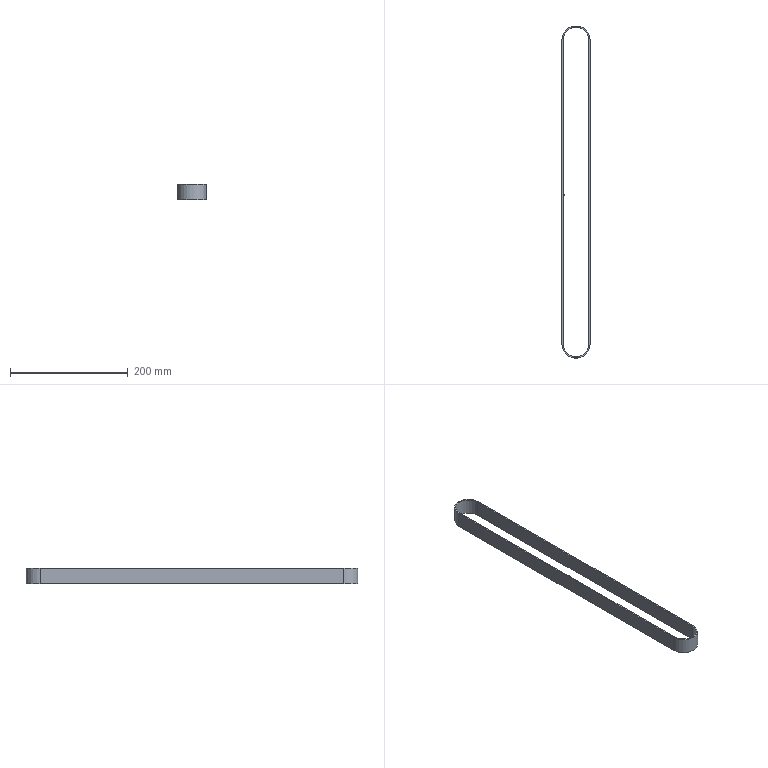Part | SolidWorks | features CompositeCurve 1, Extrusion 1, ICE 1 | 1 solid | 19 faces | box 47.9 x 564.4 x 27 mm | volume 68430 mm3 | cylinder 12 | plane 7 | commonest cylinder face diameters 0.5 x2 1.1 x2 6.55 x2 40.06 x2 43.6 x2 47.9 x2
STEP:
#1=CARTESIAN_POINT('',(-20.121,-262.156,27.));
#2=VERTEX_POINT('',#1);
#3=CARTESIAN_POINT('',(-20.132,-262.842,27.));
#4=VERTEX_POINT('',#3);
#5=CARTESIAN_POINT('',(-0.1024,-262.842,27.));
#6=DIRECTION('',(0.,0.,1.));
#7=DIRECTION('',(-1.,0.,0.));
#8=AXIS2_PLACEMENT_3D('',#5,#6,#7);
#9=CIRCLE('',#8,20.03);
#10=EDGE_CURVE('',#2,#4,#9,.T.);
#11=ORIENTED_EDGE('',*,*,#10,.T.);
#12=CARTESIAN_POINT('',(-20.132,-262.842,0.));
#13=VERTEX_POINT('',#12);
#14=CARTESIAN_POINT('',(-20.132,-262.842,31.346));
#15=DIRECTION('',(0.,0.,-1.));
#16=VECTOR('',#15,1000.);
#17=LINE('',#14,#16);
#18=EDGE_CURVE('',#4,#13,#17,.T.);
#19=ORIENTED_EDGE('',*,*,#18,.T.);
#20=CARTESIAN_POINT('',(-20.121,-262.156,0.));
#21=VERTEX_POINT('',#20);
#22=CARTESIAN_POINT('',(-0.1024,-262.842,0.));
#23=DIRECTION('',(0.,0.,-1.));
#24=DIRECTION('',(1.,0.,0.));
#25=AXIS2_PLACEMENT_3D('',#22,#23,#24);
#26=CIRCLE('',#25,20.03);
#27=EDGE_CURVE('',#13,#21,#26,.T.);
#28=ORIENTED_EDGE('',*,*,#27,.T.);
#29=CARTESIAN_POINT('',(-20.121,-262.156,31.346));
#30=DIRECTION('',(0.,0.,-1.));
#31=VECTOR('',#30,1000.);
#32=LINE('',#29,#31);
#33=EDGE_CURVE('',#2,#21,#32,.T.);
#34=ORIENTED_EDGE('',*,*,#33,.F.);
#35=EDGE_LOOP('',(#11,#19,#28,#34));
#36=FACE_OUTER_BOUND('',#35,.T.);
#37=CARTESIAN_POINT('',(-0.1024,-262.842,31.346));
#38=DIRECTION('',(0.,0.,-1.));
#39=DIRECTION('',(-1.,0.,0.));
#40=AXIS2_PLACEMENT_3D('',#37,#38,#39);
#41=CYLINDRICAL_SURFACE('',#40,20.03);
#42=ADVANCED_FACE('',(#36),#41,.F.);
#43=CARTESIAN_POINT('',(-21.8,-260.838,27.));
#44=VERTEX_POINT('',#43);
#45=CARTESIAN_POINT('',(-21.8,0.,27.));
#46=VERTEX_POINT('',#45);
#47=CARTESIAN_POINT('',(-21.8,-516.5,27.));
#48=DIRECTION('',(0.,1.,0.));
#49=VECTOR('',#48,1000.);
#50=LINE('',#47,#49);
#51=EDGE_CURVE('',#44,#46,#50,.T.);
#52=ORIENTED_EDGE('',*,*,#51,.F.);
#53=CARTESIAN_POINT('',(-21.8,-260.838,0.));
#54=VERTEX_POINT('',#53);
#55=CARTESIAN_POINT('',(-21.8,-260.838,31.346));
#56=DIRECTION('',(0.,0.,-1.));
#57=VECTOR('',#56,1000.);
#58=LINE('',#55,#57);
#59=EDGE_CURVE('',#44,#54,#58,.T.);
#60=ORIENTED_EDGE('',*,*,#59,.T.);
#61=CARTESIAN_POINT('',(-21.8,0.,0.));
#62=VERTEX_POINT('',#61);
#63=CARTESIAN_POINT('',(-21.8,-516.5,0.));
#64=DIRECTION('',(0.,-1.,0.));
#65=VECTOR('',#64,1000.);
#66=LINE('',#63,#65);
#67=EDGE_CURVE('',#62,#54,#66,.T.);
#68=ORIENTED_EDGE('',*,*,#67,.F.);
#69=CARTESIAN_POINT('',(-21.8,0.,593.429));
#70=DIRECTION('',(0.,0.,-1.));
#71=VECTOR('',#70,1000.);
#72=LINE('',#69,#71);
#73=EDGE_CURVE('',#46,#62,#72,.T.);
#74=ORIENTED_EDGE('',*,*,#73,.F.);
#75=EDGE_LOOP('',(#52,#60,#68,#74));
#76=FACE_OUTER_BOUND('',#75,.T.);
#77=CARTESIAN_POINT('',(-21.8,-516.5,593.429));
#78=DIRECTION('',(1.,0.,0.));
#79=DIRECTION('',(0.,0.,-1.));
#80=AXIS2_PLACEMENT_3D('',#77,#78,#79);
#81=PLANE('',#80);
#82=ADVANCED_FACE('',(#76),#81,.T.);
#83=CARTESIAN_POINT('',(-21.8,-264.847,0.));
#84=VERTEX_POINT('',#83);
#85=CARTESIAN_POINT('',(-21.8,-516.5,0.));
#86=VERTEX_POINT('',#85);
#87=CARTESIAN_POINT('',(-21.8,-516.5,0.));
#88=DIRECTION('',(0.,-1.,0.));
#89=VECTOR('',#88,1000.);
#90=LINE('',#87,#89);
#91=EDGE_CURVE('',#84,#86,#90,.T.);
#92=ORIENTED_EDGE('',*,*,#91,.F.);
#93=CARTESIAN_POINT('',(-21.8,-264.847,27.));
#94=VERTEX_POINT('',#93);
#95=CARTESIAN_POINT('',(-21.8,-264.847,31.346));
#96=DIRECTION('',(0.,0.,-1.));
#97=VECTOR('',#96,1000.);
#98=LINE('',#95,#97);
#99=EDGE_CURVE('',#94,#84,#98,.T.);
#100=ORIENTED_EDGE('',*,*,#99,.F.);
#101=CARTESIAN_POINT('',(-21.8,-516.5,27.));
#102=VERTEX_POINT('',#101);
#103=CARTESIAN_POINT('',(-21.8,-516.5,27.));
#104=DIRECTION('',(0.,1.,0.));
#105=VECTOR('',#104,1000.);
#106=LINE('',#103,#105);
#107=EDGE_CURVE('',#102,#94,#106,.T.);
#108=ORIENTED_EDGE('',*,*,#107,.F.);
#109=CARTESIAN_POINT('',(-21.8,-516.5,593.429));
#110=DIRECTION('',(0.,0.,-1.));
#111=VECTOR('',#110,1000.);
#112=LINE('',#109,#111);
#113=EDGE_CURVE('',#102,#86,#112,.T.);
#114=ORIENTED_EDGE('',*,*,#113,.T.);
#115=EDGE_LOOP('',(#92,#100,#108,#114));
#116=FACE_OUTER_BOUND('',#115,.T.);
#117=CARTESIAN_POINT('',(-21.8,-516.5,593.429));
#118=DIRECTION('',(1.,0.,0.));
#119=DIRECTION('',(0.,0.,-1.));
#120=AXIS2_PLACEMENT_3D('',#117,#118,#119);
#121=PLANE('',#120);
#122=ADVANCED_FACE('',(#116),#121,.T.);
#123=CARTESIAN_POINT('',(-23.95,-516.5,0.));
#124=VERTEX_POINT('',#123);
#125=CARTESIAN_POINT('',(23.95,-516.5,0.));
#126=VERTEX_POINT('',#125);
#127=CARTESIAN_POINT('',(0.,-516.5,0.));
#128=DIRECTION('',(0.,0.,1.));
#129=DIRECTION('',(1.,0.,0.));
#130=AXIS2_PLACEMENT_3D('',#127,#128,#129);
#131=CIRCLE('',#130,23.95);
#132=EDGE_CURVE('',#124,#126,#131,.T.);
#133=ORIENTED_EDGE('',*,*,#132,.F.);
#134=CARTESIAN_POINT('',(-23.95,0.,0.));
#135=VERTEX_POINT('',#134);
#136=CARTESIAN_POINT('',(-23.95,0.,0.));
#137=DIRECTION('',(0.,-1.,0.));
#138=VECTOR('',#137,1000.);
#139=LINE('',#136,#138);
#140=EDGE_CURVE('',#135,#124,#139,.T.);
#141=ORIENTED_EDGE('',*,*,#140,.F.);
#142=CARTESIAN_POINT('',(23.95,0.,0.));
#143=VERTEX_POINT('',#142);
#144=CARTESIAN_POINT('',(0.,0.,0.));
#145=DIRECTION('',(0.,0.,1.));
#146=DIRECTION('',(1.,0.,0.));
#147=AXIS2_PLACEMENT_3D('',#144,#145,#146);
#148=CIRCLE('',#147,23.95);
#149=EDGE_CURVE('',#143,#135,#148,.T.);
#150=ORIENTED_EDGE('',*,*,#149,.F.);
#151=CARTESIAN_POINT('',(23.95,-516.5,0.));
#152=DIRECTION('',(0.,1.,0.));
#153=VECTOR('',#152,1000.);
#154=LINE('',#151,#153);
#155=EDGE_CURVE('',#126,#143,#154,.T.);
#156=ORIENTED_EDGE('',*,*,#155,.F.);
#157=EDGE_LOOP('',(#133,#141,#150,#156));
#158=FACE_OUTER_BOUND('',#157,.T.);
#159=CARTESIAN_POINT('',(21.8,0.,0.));
#160=VERTEX_POINT('',#159);
#161=CARTESIAN_POINT('',(0.,0.,0.));
#162=DIRECTION('',(0.,0.,1.));
#163=DIRECTION('',(1.,0.,0.));
#164=AXIS2_PLACEMENT_3D('',#161,#162,#163);
#165=CIRCLE('',#164,21.8);
#166=EDGE_CURVE('',#160,#62,#165,.T.);
#167=ORIENTED_EDGE('',*,*,#166,.T.);
#168=ORIENTED_EDGE('',*,*,#67,.T.);
#169=CARTESIAN_POINT('',(-21.407,-261.313,0.));
#170=VERTEX_POINT('',#169);
#171=CARTESIAN_POINT('',(-21.253,-260.785,0.));
#172=DIRECTION('',(0.,0.,-1.));
#173=DIRECTION('',(1.,0.,0.));
#174=AXIS2_PLACEMENT_3D('',#171,#172,#173);
#175=CIRCLE('',#174,0.55);
#176=EDGE_CURVE('',#170,#54,#175,.T.);
#177=ORIENTED_EDGE('',*,*,#176,.F.);
#178=CARTESIAN_POINT('',(-20.209,-261.956,0.));
#179=VERTEX_POINT('',#178);
#180=CARTESIAN_POINT('',(-22.324,-264.457,0.));
#181=DIRECTION('',(0.,0.,-1.));
#182=DIRECTION('',(1.,0.,0.));
#183=AXIS2_PLACEMENT_3D('',#180,#181,#182);
#184=CIRCLE('',#183,3.275);
#185=EDGE_CURVE('',#170,#179,#184,.T.);
#186=ORIENTED_EDGE('',*,*,#185,.T.);
#187=CARTESIAN_POINT('',(-20.371,-262.147,0.));
#188=DIRECTION('',(0.,0.,-1.));
#189=DIRECTION('',(1.,0.,0.));
#190=AXIS2_PLACEMENT_3D('',#187,#188,#189);
#191=CIRCLE('',#190,0.25);
#192=EDGE_CURVE('',#179,#21,#191,.T.);
#193=ORIENTED_EDGE('',*,*,#192,.T.);
#194=ORIENTED_EDGE('',*,*,#27,.F.);
#195=CARTESIAN_POINT('',(-20.121,-263.529,0.));
#196=VERTEX_POINT('',#195);
#197=CARTESIAN_POINT('',(-0.1024,-262.842,0.));
#198=DIRECTION('',(0.,0.,-1.));
#199=DIRECTION('',(1.,0.,0.));
#200=AXIS2_PLACEMENT_3D('',#197,#198,#199);
#201=CIRCLE('',#200,20.03);
#202=EDGE_CURVE('',#196,#13,#201,.T.);
#203=ORIENTED_EDGE('',*,*,#202,.F.);
#204=CARTESIAN_POINT('',(-20.209,-263.729,0.));
#205=VERTEX_POINT('',#204);
#206=CARTESIAN_POINT('',(-20.371,-263.538,0.));
#207=DIRECTION('',(0.,0.,-1.));
#208=DIRECTION('',(1.,0.,0.));
#209=AXIS2_PLACEMENT_3D('',#206,#207,#208);
#210=CIRCLE('',#209,0.25);
#211=EDGE_CURVE('',#196,#205,#210,.T.);
#212=ORIENTED_EDGE('',*,*,#211,.T.);
#213=CARTESIAN_POINT('',(-21.407,-264.372,0.));
#214=VERTEX_POINT('',#213);
#215=CARTESIAN_POINT('',(-22.324,-261.228,0.));
#216=DIRECTION('',(0.,0.,-1.));
#217=DIRECTION('',(1.,0.,0.));
#218=AXIS2_PLACEMENT_3D('',#215,#216,#217);
#219=CIRCLE('',#218,3.275);
#220=EDGE_CURVE('',#205,#214,#219,.T.);
#221=ORIENTED_EDGE('',*,*,#220,.T.);
#222=CARTESIAN_POINT('',(-21.253,-264.9,0.));
#223=DIRECTION('',(0.,0.,-1.));
#224=DIRECTION('',(1.,0.,0.));
#225=AXIS2_PLACEMENT_3D('',#222,#223,#224);
#226=CIRCLE('',#225,0.55);
#227=EDGE_CURVE('',#84,#214,#226,.T.);
#228=ORIENTED_EDGE('',*,*,#227,.F.);
#229=ORIENTED_EDGE('',*,*,#91,.T.);
#230=CARTESIAN_POINT('',(21.8,-516.5,0.));
#231=VERTEX_POINT('',#230);
#232=CARTESIAN_POINT('',(0.,-516.5,0.));
#233=DIRECTION('',(0.,0.,1.));
#234=DIRECTION('',(1.,0.,0.));
#235=AXIS2_PLACEMENT_3D('',#232,#233,#234);
#236=CIRCLE('',#235,21.8);
#237=EDGE_CURVE('',#86,#231,#236,.T.);
#238=ORIENTED_EDGE('',*,*,#237,.T.);
#239=CARTESIAN_POINT('',(21.8,0.,0.));
#240=DIRECTION('',(0.,1.,0.));
#241=VECTOR('',#240,1000.);
#242=LINE('',#239,#241);
#243=EDGE_CURVE('',#231,#160,#242,.T.);
#244=ORIENTED_EDGE('',*,*,#243,.T.);
#245=EDGE_LOOP('',(#167,#168,#177,#186,#193,#194,#203,#212,#221,#228,#229,#238,#244));
#246=FACE_BOUND('',#245,.T.);
#247=CARTESIAN_POINT('',(0.,-516.5,0.));
#248=DIRECTION('',(0.,0.,1.));
#249=DIRECTION('',(1.,0.,0.));
#250=AXIS2_PLACEMENT_3D('',#247,#248,#249);
#251=PLANE('',#250);
#252=ADVANCED_FACE('',(#158,#246),#251,.F.);
#253=CARTESIAN_POINT('',(23.95,-516.5,27.));
#254=VERTEX_POINT('',#253);
#255=CARTESIAN_POINT('',(23.95,-516.5,593.429));
#256=DIRECTION('',(0.,0.,-1.));
#257=VECTOR('',#256,1000.);
#258=LINE('',#255,#257);
#259=EDGE_CURVE('',#254,#126,#258,.T.);
#260=ORIENTED_EDGE('',*,*,#259,.F.);
#261=CARTESIAN_POINT('',(-23.95,-516.5,27.));
#262=VERTEX_POINT('',#261);
#263=CARTESIAN_POINT('',(0.,-516.5,27.));
#264=DIRECTION('',(0.,0.,-1.));
#265=DIRECTION('',(-1.,0.,0.));
#266=AXIS2_PLACEMENT_3D('',#263,#264,#265);
#267=CIRCLE('',#266,23.95);
#268=EDGE_CURVE('',#254,#262,#267,.T.);
#269=ORIENTED_EDGE('',*,*,#268,.T.);
#270=CARTESIAN_POINT('',(-23.95,-516.5,593.429));
#271=DIRECTION('',(0.,0.,-1.));
#272=VECTOR('',#271,1000.);
#273=LINE('',#270,#272);
#274=EDGE_CURVE('',#262,#124,#273,.T.);
#275=ORIENTED_EDGE('',*,*,#274,.T.);
#276=ORIENTED_EDGE('',*,*,#132,.T.);
#277=EDGE_LOOP('',(#260,#269,#275,#276));
#278=FACE_OUTER_BOUND('',#277,.T.);
#279=CARTESIAN_POINT('',(0.,-516.5,593.429));
#280=DIRECTION('',(0.,0.,-1.));
#281=DIRECTION('',(-1.,0.,0.));
#282=AXIS2_PLACEMENT_3D('',#279,#280,#281);
#283=CYLINDRICAL_SURFACE('',#282,23.95);
#284=ADVANCED_FACE('',(#278),#283,.T.);
#285=CARTESIAN_POINT('',(23.95,0.,27.));
#286=VERTEX_POINT('',#285);
#287=CARTESIAN_POINT('',(23.95,0.,593.429));
#288=DIRECTION('',(0.,0.,-1.));
#289=VECTOR('',#288,1000.);
#290=LINE('',#287,#289);
#291=EDGE_CURVE('',#286,#143,#290,.T.);
#292=ORIENTED_EDGE('',*,*,#291,.F.);
#293=CARTESIAN_POINT('',(23.95,-516.5,27.));
#294=DIRECTION('',(0.,-1.,0.));
#295=VECTOR('',#294,1000.);
#296=LINE('',#293,#295);
#297=EDGE_CURVE('',#286,#254,#296,.T.);
#298=ORIENTED_EDGE('',*,*,#297,.T.);
#299=ORIENTED_EDGE('',*,*,#259,.T.);
#300=ORIENTED_EDGE('',*,*,#155,.T.);
#301=EDGE_LOOP('',(#292,#298,#299,#300));
#302=FACE_OUTER_BOUND('',#301,.T.);
#303=CARTESIAN_POINT('',(23.95,-516.5,593.429));
#304=DIRECTION('',(-1.,0.,0.));
#305=DIRECTION('',(0.,-1.,0.));
#306=AXIS2_PLACEMENT_3D('',#303,#304,#305);
#307=PLANE('',#306);
#308=ADVANCED_FACE('',(#302),#307,.F.);
#309=CARTESIAN_POINT('',(-23.95,0.,27.));
#310=VERTEX_POINT('',#309);
#311=CARTESIAN_POINT('',(-23.95,0.,593.429));
#312=DIRECTION('',(0.,0.,-1.));
#313=VECTOR('',#312,1000.);
#314=LINE('',#311,#313);
#315=EDGE_CURVE('',#310,#135,#314,.T.);
#316=ORIENTED_EDGE('',*,*,#315,.F.);
#317=CARTESIAN_POINT('',(0.,0.,27.));
#318=DIRECTION('',(0.,0.,-1.));
#319=DIRECTION('',(-1.,0.,0.));
#320=AXIS2_PLACEMENT_3D('',#317,#318,#319);
#321=CIRCLE('',#320,23.95);
#322=EDGE_CURVE('',#310,#286,#321,.T.);
#323=ORIENTED_EDGE('',*,*,#322,.T.);
#324=ORIENTED_EDGE('',*,*,#291,.T.);
#325=ORIENTED_EDGE('',*,*,#149,.T.);
#326=EDGE_LOOP('',(#316,#323,#324,#325));
#327=FACE_OUTER_BOUND('',#326,.T.);
#328=CARTESIAN_POINT('',(0.,0.,593.429));
#329=DIRECTION('',(0.,0.,-1.));
#330=DIRECTION('',(-1.,0.,0.));
#331=AXIS2_PLACEMENT_3D('',#328,#329,#330);
#332=CYLINDRICAL_SURFACE('',#331,23.95);
#333=ADVANCED_FACE('',(#327),#332,.T.);
#334=ORIENTED_EDGE('',*,*,#274,.F.);
#335=CARTESIAN_POINT('',(-23.95,0.,27.));
#336=DIRECTION('',(0.,1.,0.));
#337=VECTOR('',#336,1000.);
#338=LINE('',#335,#337);
#339=EDGE_CURVE('',#262,#310,#338,.T.);
#340=ORIENTED_EDGE('',*,*,#339,.T.);
#341=ORIENTED_EDGE('',*,*,#315,.T.);
#342=ORIENTED_EDGE('',*,*,#140,.T.);
#343=EDGE_LOOP('',(#334,#340,#341,#342));
#344=FACE_OUTER_BOUND('',#343,.T.);
#345=CARTESIAN_POINT('',(-23.95,0.,593.429));
#346=DIRECTION('',(1.,0.,0.));
#347=DIRECTION('',(0.,1.,0.));
#348=AXIS2_PLACEMENT_3D('',#345,#346,#347);
#349=PLANE('',#348);
#350=ADVANCED_FACE('',(#344),#349,.F.);
#351=CARTESIAN_POINT('',(21.8,0.,27.));
#352=VERTEX_POINT('',#351);
#353=CARTESIAN_POINT('',(0.,0.,27.));
#354=DIRECTION('',(0.,0.,-1.));
#355=DIRECTION('',(-1.,0.,0.));
#356=AXIS2_PLACEMENT_3D('',#353,#354,#355);
#357=CIRCLE('',#356,21.8);
#358=EDGE_CURVE('',#46,#352,#357,.T.);
#359=ORIENTED_EDGE('',*,*,#358,.F.);
#360=ORIENTED_EDGE('',*,*,#73,.T.);
#361=ORIENTED_EDGE('',*,*,#166,.F.);
#362=CARTESIAN_POINT('',(21.8,0.,593.429));
#363=DIRECTION('',(0.,0.,-1.));
#364=VECTOR('',#363,1000.);
#365=LINE('',#362,#364);
#366=EDGE_CURVE('',#352,#160,#365,.T.);
#367=ORIENTED_EDGE('',*,*,#366,.F.);
#368=EDGE_LOOP('',(#359,#360,#361,#367));
#369=FACE_OUTER_BOUND('',#368,.T.);
#370=CARTESIAN_POINT('',(0.,0.,593.429));
#371=DIRECTION('',(0.,0.,-1.));
#372=DIRECTION('',(-1.,0.,0.));
#373=AXIS2_PLACEMENT_3D('',#370,#371,#372);
#374=CYLINDRICAL_SURFACE('',#373,21.8);
#375=ADVANCED_FACE('',(#369),#374,.F.);
#376=CARTESIAN_POINT('',(21.8,-516.5,27.));
#377=VERTEX_POINT('',#376);
#378=CARTESIAN_POINT('',(0.,-516.5,27.));
#379=DIRECTION('',(0.,0.,-1.));
#380=DIRECTION('',(-1.,0.,0.));
#381=AXIS2_PLACEMENT_3D('',#378,#379,#380);
#382=CIRCLE('',#381,21.8);
#383=EDGE_CURVE('',#377,#102,#382,.T.);
#384=ORIENTED_EDGE('',*,*,#383,.F.);
#385=CARTESIAN_POINT('',(21.8,-516.5,593.429));
#386=DIRECTION('',(0.,0.,-1.));
#387=VECTOR('',#386,1000.);
#388=LINE('',#385,#387);
#389=EDGE_CURVE('',#377,#231,#388,.T.);
#390=ORIENTED_EDGE('',*,*,#389,.T.);
#391=ORIENTED_EDGE('',*,*,#237,.F.);
#392=ORIENTED_EDGE('',*,*,#113,.F.);
#393=EDGE_LOOP('',(#384,#390,#391,#392));
#394=FACE_OUTER_BOUND('',#393,.T.);
#395=CARTESIAN_POINT('',(0.,-516.5,593.429));
#396=DIRECTION('',(0.,0.,-1.));
#397=DIRECTION('',(-1.,0.,0.));
#398=AXIS2_PLACEMENT_3D('',#395,#396,#397);
#399=CYLINDRICAL_SURFACE('',#398,21.8);
#400=ADVANCED_FACE('',(#394),#399,.F.);
#401=CARTESIAN_POINT('',(21.8,0.,27.));
#402=DIRECTION('',(0.,-1.,0.));
#403=VECTOR('',#402,1000.);
#404=LINE('',#401,#403);
#405=EDGE_CURVE('',#352,#377,#404,.T.);
#406=ORIENTED_EDGE('',*,*,#405,.F.);
#407=ORIENTED_EDGE('',*,*,#366,.T.);
#408=ORIENTED_EDGE('',*,*,#243,.F.);
#409=ORIENTED_EDGE('',*,*,#389,.F.);
#410=EDGE_LOOP('',(#406,#407,#408,#409));
#411=FACE_OUTER_BOUND('',#410,.T.);
#412=CARTESIAN_POINT('',(21.8,0.,593.429));
#413=DIRECTION('',(-1.,0.,0.));
#414=DIRECTION('',(0.,0.,1.));
#415=AXIS2_PLACEMENT_3D('',#412,#413,#414);
#416=PLANE('',#415);
#417=ADVANCED_FACE('',(#411),#416,.T.);
#418=ORIENTED_EDGE('',*,*,#358,.T.);
#419=ORIENTED_EDGE('',*,*,#405,.T.);
#420=ORIENTED_EDGE('',*,*,#383,.T.);
#421=ORIENTED_EDGE('',*,*,#107,.T.);
#422=CARTESIAN_POINT('',(-21.407,-264.372,27.));
#423=VERTEX_POINT('',#422);
#424=CARTESIAN_POINT('',(-21.253,-264.9,27.));
#425=DIRECTION('',(0.,0.,1.));
#426=DIRECTION('',(-1.,0.,0.));
#427=AXIS2_PLACEMENT_3D('',#424,#425,#426);
#428=CIRCLE('',#427,0.55);
#429=EDGE_CURVE('',#423,#94,#428,.T.);
#430=ORIENTED_EDGE('',*,*,#429,.F.);
#431=CARTESIAN_POINT('',(-20.209,-263.729,27.));
#432=VERTEX_POINT('',#431);
#433=CARTESIAN_POINT('',(-22.324,-261.228,27.));
#434=DIRECTION('',(0.,0.,1.));
#435=DIRECTION('',(-1.,0.,0.));
#436=AXIS2_PLACEMENT_3D('',#433,#434,#435);
#437=CIRCLE('',#436,3.275);
#438=EDGE_CURVE('',#423,#432,#437,.T.);
#439=ORIENTED_EDGE('',*,*,#438,.T.);
#440=CARTESIAN_POINT('',(-20.121,-263.529,27.));
#441=VERTEX_POINT('',#440);
#442=CARTESIAN_POINT('',(-20.371,-263.538,27.));
#443=DIRECTION('',(0.,0.,1.));
#444=DIRECTION('',(-1.,0.,0.));
#445=AXIS2_PLACEMENT_3D('',#442,#443,#444);
#446=CIRCLE('',#445,0.25);
#447=EDGE_CURVE('',#432,#441,#446,.T.);
#448=ORIENTED_EDGE('',*,*,#447,.T.);
#449=CARTESIAN_POINT('',(-0.1024,-262.842,27.));
#450=DIRECTION('',(0.,0.,1.));
#451=DIRECTION('',(-1.,0.,0.));
#452=AXIS2_PLACEMENT_3D('',#449,#450,#451);
#453=CIRCLE('',#452,20.03);
#454=EDGE_CURVE('',#4,#441,#453,.T.);
#455=ORIENTED_EDGE('',*,*,#454,.F.);
#456=ORIENTED_EDGE('',*,*,#10,.F.);
#457=CARTESIAN_POINT('',(-20.209,-261.956,27.));
#458=VERTEX_POINT('',#457);
#459=CARTESIAN_POINT('',(-20.371,-262.147,27.));
#460=DIRECTION('',(0.,0.,1.));
#461=DIRECTION('',(-1.,0.,0.));
#462=AXIS2_PLACEMENT_3D('',#459,#460,#461);
#463=CIRCLE('',#462,0.25);
#464=EDGE_CURVE('',#2,#458,#463,.T.);
#465=ORIENTED_EDGE('',*,*,#464,.T.);
#466=CARTESIAN_POINT('',(-21.407,-261.313,27.));
#467=VERTEX_POINT('',#466);
#468=CARTESIAN_POINT('',(-22.324,-264.457,27.));
#469=DIRECTION('',(0.,0.,1.));
#470=DIRECTION('',(-1.,0.,0.));
#471=AXIS2_PLACEMENT_3D('',#468,#469,#470);
#472=CIRCLE('',#471,3.275);
#473=EDGE_CURVE('',#458,#467,#472,.T.);
#474=ORIENTED_EDGE('',*,*,#473,.T.);
#475=CARTESIAN_POINT('',(-21.253,-260.785,27.));
#476=DIRECTION('',(0.,0.,1.));
#477=DIRECTION('',(-1.,0.,0.));
#478=AXIS2_PLACEMENT_3D('',#475,#476,#477);
#479=CIRCLE('',#478,0.55);
#480=EDGE_CURVE('',#44,#467,#479,.T.);
#481=ORIENTED_EDGE('',*,*,#480,.F.);
#482=ORIENTED_EDGE('',*,*,#51,.T.);
#483=EDGE_LOOP('',(#418,#419,#420,#421,#430,#439,#448,#455,#456,#465,#474,#481,#482));
#484=FACE_BOUND('',#483,.T.);
#485=ORIENTED_EDGE('',*,*,#297,.F.);
#486=ORIENTED_EDGE('',*,*,#322,.F.);
#487=ORIENTED_EDGE('',*,*,#339,.F.);
#488=ORIENTED_EDGE('',*,*,#268,.F.);
#489=EDGE_LOOP('',(#485,#486,#487,#488));
#490=FACE_OUTER_BOUND('',#489,.T.);
#491=CARTESIAN_POINT('',(0.,22.28,27.));
#492=DIRECTION('',(0.,0.,-1.));
#493=DIRECTION('',(0.,-1.,0.));
#494=AXIS2_PLACEMENT_3D('',#491,#492,#493);
#495=PLANE('',#494);
#496=ADVANCED_FACE('',(#484,#490),#495,.F.);
#497=ORIENTED_EDGE('',*,*,#59,.F.);
#498=ORIENTED_EDGE('',*,*,#480,.T.);
#499=CARTESIAN_POINT('',(-21.407,-261.313,31.346));
#500=DIRECTION('',(0.,0.,-1.));
#501=VECTOR('',#500,1000.);
#502=LINE('',#499,#501);
#503=EDGE_CURVE('',#467,#170,#502,.T.);
#504=ORIENTED_EDGE('',*,*,#503,.T.);
#505=ORIENTED_EDGE('',*,*,#176,.T.);
#506=EDGE_LOOP('',(#497,#498,#504,#505));
#507=FACE_OUTER_BOUND('',#506,.T.);
#508=CARTESIAN_POINT('',(-21.253,-260.785,31.346));
#509=DIRECTION('',(0.,0.,-1.));
#510=DIRECTION('',(-1.,0.,0.));
#511=AXIS2_PLACEMENT_3D('',#508,#509,#510);
#512=CYLINDRICAL_SURFACE('',#511,0.55);
#513=ADVANCED_FACE('',(#507),#512,.F.);
#514=ORIENTED_EDGE('',*,*,#473,.F.);
#515=CARTESIAN_POINT('',(-20.209,-261.956,31.346));
#516=DIRECTION('',(0.,0.,-1.));
#517=VECTOR('',#516,1000.);
#518=LINE('',#515,#517);
#519=EDGE_CURVE('',#458,#179,#518,.T.);
#520=ORIENTED_EDGE('',*,*,#519,.T.);
#521=ORIENTED_EDGE('',*,*,#185,.F.);
#522=ORIENTED_EDGE('',*,*,#503,.F.);
#523=EDGE_LOOP('',(#514,#520,#521,#522));
#524=FACE_OUTER_BOUND('',#523,.T.);
#525=CARTESIAN_POINT('',(-22.324,-264.457,31.346));
#526=DIRECTION('',(0.,0.,-1.));
#527=DIRECTION('',(-1.,0.,0.));
#528=AXIS2_PLACEMENT_3D('',#525,#526,#527);
#529=CYLINDRICAL_SURFACE('',#528,3.275);
#530=ADVANCED_FACE('',(#524),#529,.T.);
#531=ORIENTED_EDGE('',*,*,#464,.F.);
#532=ORIENTED_EDGE('',*,*,#33,.T.);
#533=ORIENTED_EDGE('',*,*,#192,.F.);
#534=ORIENTED_EDGE('',*,*,#519,.F.);
#535=EDGE_LOOP('',(#531,#532,#533,#534));
#536=FACE_OUTER_BOUND('',#535,.T.);
#537=CARTESIAN_POINT('',(-20.371,-262.147,31.346));
#538=DIRECTION('',(0.,0.,-1.));
#539=DIRECTION('',(-1.,0.,0.));
#540=AXIS2_PLACEMENT_3D('',#537,#538,#539);
#541=CYLINDRICAL_SURFACE('',#540,0.25);
#542=ADVANCED_FACE('',(#536),#541,.T.);
#543=ORIENTED_EDGE('',*,*,#18,.F.);
#544=ORIENTED_EDGE('',*,*,#454,.T.);
#545=CARTESIAN_POINT('',(-20.121,-263.529,31.346));
#546=DIRECTION('',(0.,0.,-1.));
#547=VECTOR('',#546,1000.);
#548=LINE('',#545,#547);
#549=EDGE_CURVE('',#441,#196,#548,.T.);
#550=ORIENTED_EDGE('',*,*,#549,.T.);
#551=ORIENTED_EDGE('',*,*,#202,.T.);
#552=EDGE_LOOP('',(#543,#544,#550,#551));
#553=FACE_OUTER_BOUND('',#552,.T.);
#554=CARTESIAN_POINT('',(-0.1024,-262.842,31.346));
#555=DIRECTION('',(0.,0.,-1.));
#556=DIRECTION('',(-1.,0.,0.));
#557=AXIS2_PLACEMENT_3D('',#554,#555,#556);
#558=CYLINDRICAL_SURFACE('',#557,20.03);
#559=ADVANCED_FACE('',(#553),#558,.F.);
#560=ORIENTED_EDGE('',*,*,#447,.F.);
#561=CARTESIAN_POINT('',(-20.209,-263.729,31.346));
#562=DIRECTION('',(0.,0.,-1.));
#563=VECTOR('',#562,1000.);
#564=LINE('',#561,#563);
#565=EDGE_CURVE('',#432,#205,#564,.T.);
#566=ORIENTED_EDGE('',*,*,#565,.T.);
#567=ORIENTED_EDGE('',*,*,#211,.F.);
#568=ORIENTED_EDGE('',*,*,#549,.F.);
#569=EDGE_LOOP('',(#560,#566,#567,#568));
#570=FACE_OUTER_BOUND('',#569,.T.);
#571=CARTESIAN_POINT('',(-20.371,-263.538,31.346));
#572=DIRECTION('',(0.,0.,-1.));
#573=DIRECTION('',(-1.,0.,0.));
#574=AXIS2_PLACEMENT_3D('',#571,#572,#573);
#575=CYLINDRICAL_SURFACE('',#574,0.25);
#576=ADVANCED_FACE('',(#570),#575,.T.);
#577=ORIENTED_EDGE('',*,*,#438,.F.);
#578=CARTESIAN_POINT('',(-21.407,-264.372,31.346));
#579=DIRECTION('',(0.,0.,-1.));
#580=VECTOR('',#579,1000.);
#581=LINE('',#578,#580);
#582=EDGE_CURVE('',#423,#214,#581,.T.);
#583=ORIENTED_EDGE('',*,*,#582,.T.);
#584=ORIENTED_EDGE('',*,*,#220,.F.);
#585=ORIENTED_EDGE('',*,*,#565,.F.);
#586=EDGE_LOOP('',(#577,#583,#584,#585));
#587=FACE_OUTER_BOUND('',#586,.T.);
#588=CARTESIAN_POINT('',(-22.324,-261.228,31.346));
#589=DIRECTION('',(0.,0.,-1.));
#590=DIRECTION('',(-1.,0.,0.));
#591=AXIS2_PLACEMENT_3D('',#588,#589,#590);
#592=CYLINDRICAL_SURFACE('',#591,3.275);
#593=ADVANCED_FACE('',(#587),#592,.T.);
#594=ORIENTED_EDGE('',*,*,#582,.F.);
#595=ORIENTED_EDGE('',*,*,#429,.T.);
#596=ORIENTED_EDGE('',*,*,#99,.T.);
#597=ORIENTED_EDGE('',*,*,#227,.T.);
#598=EDGE_LOOP('',(#594,#595,#596,#597));
#599=FACE_OUTER_BOUND('',#598,.T.);
#600=CARTESIAN_POINT('',(-21.253,-264.9,31.346));
#601=DIRECTION('',(0.,0.,-1.));
#602=DIRECTION('',(-1.,0.,0.));
#603=AXIS2_PLACEMENT_3D('',#600,#601,#602);
#604=CYLINDRICAL_SURFACE('',#603,0.55);
#605=ADVANCED_FACE('',(#599),#604,.F.);
#606=CLOSED_SHELL('',(#42,#82,#122,#252,#284,#308,#333,#350,#375,#400,#417,#496,#513,#530,#542,#559,#576,#593,#605));
#607=MANIFOLD_SOLID_BREP('',#606);
#608=CARTESIAN_POINT('',(0.,0.,0.));
#609=DIRECTION('',(0.,0.,1.));
#610=DIRECTION('',(1.,0.,0.));
#611=AXIS2_PLACEMENT_3D('',#608,#609,#610);
#612=(LENGTH_UNIT()NAMED_UNIT(*)SI_UNIT(.MILLI.,.METRE.));
#613=UNCERTAINTY_MEASURE_WITH_UNIT(LENGTH_MEASURE(0.00001),#612,'','');
#614=(NAMED_UNIT(*)PLANE_ANGLE_UNIT()SI_UNIT($,.RADIAN.));
#615=(NAMED_UNIT(*)SI_UNIT($,.STERADIAN.)SOLID_ANGLE_UNIT());
#616=(GEOMETRIC_REPRESENTATION_CONTEXT(3)GLOBAL_UNCERTAINTY_ASSIGNED_CONTEXT((#613))GLOBAL_UNIT_ASSIGNED_CONTEXT((#612,#614,#615))REPRESENTATION_CONTEXT('',''));
#617=ADVANCED_BREP_SHAPE_REPRESENTATION('',(#607,#611),#616);